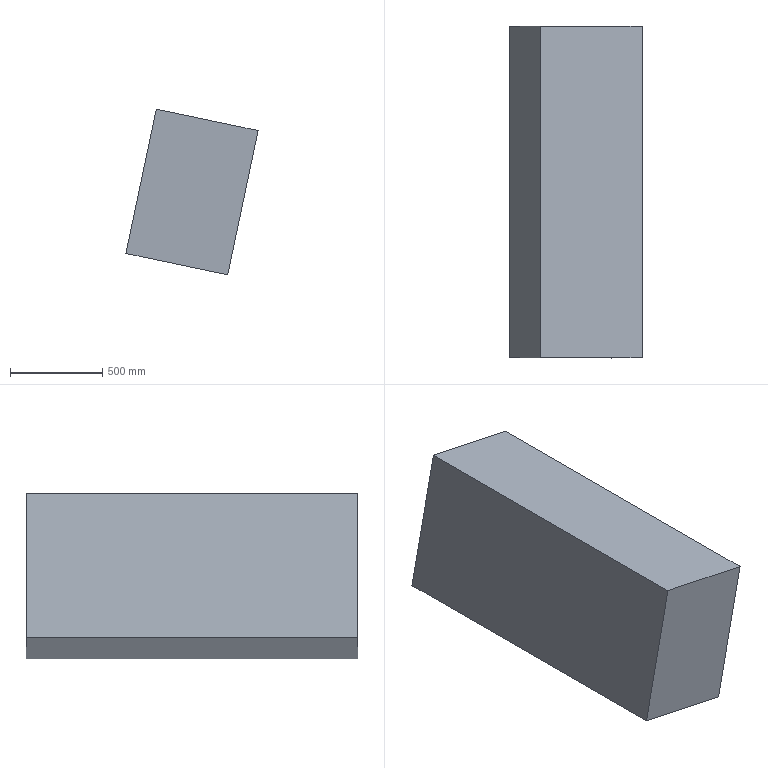Part | STEP file | 5_ESTAGIO_MAQUINA | 1 solid | 6 faces | box 717.439 x 1800 x 899.09 mm | volume 813600000 mm3 | plane 6
STEP:
#1=CARTESIAN_POINT('',(0.,0.,0.));
#2=DIRECTION('',(0.,0.,1.));
#3=DIRECTION('',(1.,0.,0.));
#4=AXIS2_PLACEMENT_3D('',#1,#2,#3);
#5=CARTESIAN_POINT('',(-2622.628,266.85,-322.944));
#6=VERTEX_POINT('',#5);
#7=CARTESIAN_POINT('',(-3175.552,266.85,-206.755));
#8=VERTEX_POINT('',#7);
#9=CARTESIAN_POINT('',(-2622.628,266.85,-322.944));
#10=DIRECTION('',(-0.9786,0.,0.2056));
#11=VECTOR('',#10,1.);
#12=LINE('',#9,#11);
#13=CARTESIAN_POINT('',(-2458.113,266.85,459.958));
#14=DIRECTION('',(0.,-1.,0.));
#15=DIRECTION('',(0.,0.,-1.));
#16=AXIS2_PLACEMENT_3D('',#13,#14,#15);
#17=PLANE('',#16);
#18=CARTESIAN_POINT('',(782.902,-164.515));
#19=DIRECTION('',(-0.2056,-0.9786));
#20=VECTOR('',#19,1.);
#21=LINE('',#18,#20);
#22=(GEOMETRIC_REPRESENTATION_CONTEXT(2)PARAMETRIC_REPRESENTATION_CONTEXT()REPRESENTATION_CONTEXT('',''));
#23=DEFINITIONAL_REPRESENTATION('',(#21),#22);
#24=PCURVE('',#17,#23);
#25=CARTESIAN_POINT('',(-175.901,0.,-837.086));
#26=DIRECTION('',(0.2056,0.,0.9786));
#27=DIRECTION('',(0.9786,0.,-0.2056));
#28=AXIS2_PLACEMENT_3D('',#25,#26,#27);
#29=PLANE('',#28);
#30=CARTESIAN_POINT('',(-2500.163,266.85));
#31=DIRECTION('',(-1.,0.));
#32=VECTOR('',#31,1.);
#33=LINE('',#30,#32);
#34=(GEOMETRIC_REPRESENTATION_CONTEXT(2)PARAMETRIC_REPRESENTATION_CONTEXT()REPRESENTATION_CONTEXT('',''));
#35=DEFINITIONAL_REPRESENTATION('',(#33),#34);
#36=PCURVE('',#29,#35);
#37=SURFACE_CURVE('',#12,(#24,#36),.PCURVE_S1.);
#38=EDGE_CURVE('',#6,#8,#37,.T.);
#39=ORIENTED_EDGE('',*,*,#38,.T.);
#40=CARTESIAN_POINT('',(-3011.037,266.85,576.146));
#41=VERTEX_POINT('',#40);
#42=CARTESIAN_POINT('',(-3011.037,266.85,576.146));
#43=DIRECTION('',(-0.2056,0.,-0.9786));
#44=VECTOR('',#43,1.);
#45=LINE('',#42,#44);
#46=CARTESIAN_POINT('',(-116.188,-552.924));
#47=DIRECTION('',(0.9786,-0.2056));
#48=VECTOR('',#47,1.);
#49=LINE('',#46,#48);
#50=(GEOMETRIC_REPRESENTATION_CONTEXT(2)PARAMETRIC_REPRESENTATION_CONTEXT()REPRESENTATION_CONTEXT('',''));
#51=DEFINITIONAL_REPRESENTATION('',(#49),#50);
#52=PCURVE('',#17,#51);
#53=CARTESIAN_POINT('',(-3011.037,-1533.15,576.146));
#54=DIRECTION('',(-0.9786,0.,0.2056));
#55=DIRECTION('',(0.2056,0.,0.9786));
#56=AXIS2_PLACEMENT_3D('',#53,#54,#55);
#57=PLANE('',#56);
#58=CARTESIAN_POINT('',(0.,1800.));
#59=DIRECTION('',(-1.,0.));
#60=VECTOR('',#59,1.);
#61=LINE('',#58,#60);
#62=(GEOMETRIC_REPRESENTATION_CONTEXT(2)PARAMETRIC_REPRESENTATION_CONTEXT()REPRESENTATION_CONTEXT('',''));
#63=DEFINITIONAL_REPRESENTATION('',(#61),#62);
#64=PCURVE('',#57,#63);
#65=SURFACE_CURVE('',#45,(#52,#64),.PCURVE_S1.);
#66=EDGE_CURVE('',#41,#8,#65,.T.);
#67=ORIENTED_EDGE('',*,*,#66,.F.);
#68=CARTESIAN_POINT('',(-2458.113,266.85,459.958));
#69=VERTEX_POINT('',#68);
#70=CARTESIAN_POINT('',(-2458.113,266.85,459.958));
#71=DIRECTION('',(-0.9786,0.,0.2056));
#72=VECTOR('',#71,1.);
#73=LINE('',#70,#72);
#74=CARTESIAN_POINT('',(0.000000001,-0.000000001));
#75=DIRECTION('',(-0.2056,-0.9786));
#76=VECTOR('',#75,1.);
#77=LINE('',#74,#76);
#78=(GEOMETRIC_REPRESENTATION_CONTEXT(2)PARAMETRIC_REPRESENTATION_CONTEXT()REPRESENTATION_CONTEXT('',''));
#79=DEFINITIONAL_REPRESENTATION('',(#77),#78);
#80=PCURVE('',#17,#79);
#81=CARTESIAN_POINT('',(-11.386,0.,-54.184));
#82=DIRECTION('',(0.2056,0.,0.9786));
#83=DIRECTION('',(0.9786,0.,-0.2056));
#84=AXIS2_PLACEMENT_3D('',#81,#82,#83);
#85=PLANE('',#84);
#86=CARTESIAN_POINT('',(-2500.163,266.85));
#87=DIRECTION('',(-1.,0.));
#88=VECTOR('',#87,1.);
#89=LINE('',#86,#88);
#90=(GEOMETRIC_REPRESENTATION_CONTEXT(2)PARAMETRIC_REPRESENTATION_CONTEXT()REPRESENTATION_CONTEXT('',''));
#91=DEFINITIONAL_REPRESENTATION('',(#89),#90);
#92=PCURVE('',#85,#91);
#93=SURFACE_CURVE('',#73,(#80,#92),.PCURVE_S1.);
#94=EDGE_CURVE('',#69,#41,#93,.T.);
#95=ORIENTED_EDGE('',*,*,#94,.F.);
#96=CARTESIAN_POINT('',(-2458.113,266.85,459.958));
#97=DIRECTION('',(-0.2056,0.,-0.9786));
#98=VECTOR('',#97,1.);
#99=LINE('',#96,#98);
#100=CARTESIAN_POINT('',(0.,-0.000000003));
#101=DIRECTION('',(0.9786,-0.2056));
#102=VECTOR('',#101,1.);
#103=LINE('',#100,#102);
#104=(GEOMETRIC_REPRESENTATION_CONTEXT(2)PARAMETRIC_REPRESENTATION_CONTEXT()REPRESENTATION_CONTEXT('',''));
#105=DEFINITIONAL_REPRESENTATION('',(#103),#104);
#106=PCURVE('',#17,#105);
#107=CARTESIAN_POINT('',(-2458.113,266.85,459.958));
#108=DIRECTION('',(0.9786,0.,-0.2056));
#109=DIRECTION('',(-0.2056,0.,-0.9786));
#110=AXIS2_PLACEMENT_3D('',#107,#108,#109);
#111=PLANE('',#110);
#112=CARTESIAN_POINT('',(0.000000001,0.));
#113=DIRECTION('',(1.,0.));
#114=VECTOR('',#113,1.);
#115=LINE('',#112,#114);
#116=(GEOMETRIC_REPRESENTATION_CONTEXT(2)PARAMETRIC_REPRESENTATION_CONTEXT()REPRESENTATION_CONTEXT('',''));
#117=DEFINITIONAL_REPRESENTATION('',(#115),#116);
#118=PCURVE('',#111,#117);
#119=SURFACE_CURVE('',#99,(#106,#118),.PCURVE_S1.);
#120=EDGE_CURVE('',#69,#6,#119,.T.);
#121=ORIENTED_EDGE('',*,*,#120,.T.);
#122=EDGE_LOOP('',(#39,#67,#95,#121));
#123=FACE_BOUND('',#122,.T.);
#124=ADVANCED_FACE('',(#123),#17,.F.);
#125=CARTESIAN_POINT('',(-3175.552,-1533.15,-206.755));
#126=VERTEX_POINT('',#125);
#127=CARTESIAN_POINT('',(-3175.552,-1533.15,-206.755));
#128=DIRECTION('',(0.,1.,0.));
#129=VECTOR('',#128,1.);
#130=LINE('',#127,#129);
#131=CARTESIAN_POINT('',(-800.,0.));
#132=DIRECTION('',(0.,1.));
#133=VECTOR('',#132,1.);
#134=LINE('',#131,#133);
#135=(GEOMETRIC_REPRESENTATION_CONTEXT(2)PARAMETRIC_REPRESENTATION_CONTEXT()REPRESENTATION_CONTEXT('',''));
#136=DEFINITIONAL_REPRESENTATION('',(#134),#135);
#137=PCURVE('',#57,#136);
#138=CARTESIAN_POINT('',(-3065.163,-1533.15));
#139=DIRECTION('',(0.,1.));
#140=VECTOR('',#139,1.);
#141=LINE('',#138,#140);
#142=(GEOMETRIC_REPRESENTATION_CONTEXT(2)PARAMETRIC_REPRESENTATION_CONTEXT()REPRESENTATION_CONTEXT('',''));
#143=DEFINITIONAL_REPRESENTATION('',(#141),#142);
#144=PCURVE('',#29,#143);
#145=SURFACE_CURVE('',#130,(#137,#144),.PCURVE_S1.);
#146=EDGE_CURVE('',#126,#8,#145,.T.);
#147=ORIENTED_EDGE('',*,*,#146,.F.);
#148=CARTESIAN_POINT('',(-3011.037,-1533.15,576.146));
#149=VERTEX_POINT('',#148);
#150=CARTESIAN_POINT('',(-3011.037,-1533.15,576.146));
#151=DIRECTION('',(-0.2056,0.,-0.9786));
#152=VECTOR('',#151,1.);
#153=LINE('',#150,#152);
#154=CARTESIAN_POINT('',(0.,0.));
#155=DIRECTION('',(-1.,0.));
#156=VECTOR('',#155,1.);
#157=LINE('',#154,#156);
#158=(GEOMETRIC_REPRESENTATION_CONTEXT(2)PARAMETRIC_REPRESENTATION_CONTEXT()REPRESENTATION_CONTEXT('',''));
#159=DEFINITIONAL_REPRESENTATION('',(#157),#158);
#160=PCURVE('',#57,#159);
#161=CARTESIAN_POINT('',(-3011.037,-1533.15,576.146));
#162=DIRECTION('',(0.,1.,0.));
#163=DIRECTION('',(0.,0.,1.));
#164=AXIS2_PLACEMENT_3D('',#161,#162,#163);
#165=PLANE('',#164);
#166=CARTESIAN_POINT('',(0.,-0.000000003));
#167=DIRECTION('',(-0.9786,-0.2056));
#168=VECTOR('',#167,1.);
#169=LINE('',#166,#168);
#170=(GEOMETRIC_REPRESENTATION_CONTEXT(2)PARAMETRIC_REPRESENTATION_CONTEXT()REPRESENTATION_CONTEXT('',''));
#171=DEFINITIONAL_REPRESENTATION('',(#169),#170);
#172=PCURVE('',#165,#171);
#173=SURFACE_CURVE('',#153,(#160,#172),.PCURVE_S1.);
#174=EDGE_CURVE('',#149,#126,#173,.T.);
#175=ORIENTED_EDGE('',*,*,#174,.F.);
#176=CARTESIAN_POINT('',(-3011.037,-1533.15,576.146));
#177=DIRECTION('',(0.,1.,0.));
#178=VECTOR('',#177,1.);
#179=LINE('',#176,#178);
#180=CARTESIAN_POINT('',(0.,0.));
#181=DIRECTION('',(0.,1.));
#182=VECTOR('',#181,1.);
#183=LINE('',#180,#182);
#184=(GEOMETRIC_REPRESENTATION_CONTEXT(2)PARAMETRIC_REPRESENTATION_CONTEXT()REPRESENTATION_CONTEXT('',''));
#185=DEFINITIONAL_REPRESENTATION('',(#183),#184);
#186=PCURVE('',#57,#185);
#187=CARTESIAN_POINT('',(-3065.163,-1533.15));
#188=DIRECTION('',(0.,1.));
#189=VECTOR('',#188,1.);
#190=LINE('',#187,#189);
#191=(GEOMETRIC_REPRESENTATION_CONTEXT(2)PARAMETRIC_REPRESENTATION_CONTEXT()REPRESENTATION_CONTEXT('',''));
#192=DEFINITIONAL_REPRESENTATION('',(#190),#191);
#193=PCURVE('',#85,#192);
#194=SURFACE_CURVE('',#179,(#186,#193),.PCURVE_S1.);
#195=EDGE_CURVE('',#149,#41,#194,.T.);
#196=ORIENTED_EDGE('',*,*,#195,.T.);
#197=ORIENTED_EDGE('',*,*,#66,.T.);
#198=EDGE_LOOP('',(#147,#175,#196,#197));
#199=FACE_BOUND('',#198,.T.);
#200=ADVANCED_FACE('',(#199),#57,.T.);
#201=CARTESIAN_POINT('',(-2622.628,-1533.15,-322.944));
#202=VERTEX_POINT('',#201);
#203=CARTESIAN_POINT('',(-3175.552,-1533.15,-206.755));
#204=DIRECTION('',(0.9786,0.,-0.2056));
#205=VECTOR('',#204,1.);
#206=LINE('',#203,#205);
#207=CARTESIAN_POINT('',(-782.902,-164.515));
#208=DIRECTION('',(-0.2056,0.9786));
#209=VECTOR('',#208,1.);
#210=LINE('',#207,#209);
#211=(GEOMETRIC_REPRESENTATION_CONTEXT(2)PARAMETRIC_REPRESENTATION_CONTEXT()REPRESENTATION_CONTEXT('',''));
#212=DEFINITIONAL_REPRESENTATION('',(#210),#211);
#213=PCURVE('',#165,#212);
#214=CARTESIAN_POINT('',(-3065.163,-1533.15));
#215=DIRECTION('',(1.,0.));
#216=VECTOR('',#215,1.);
#217=LINE('',#214,#216);
#218=(GEOMETRIC_REPRESENTATION_CONTEXT(2)PARAMETRIC_REPRESENTATION_CONTEXT()REPRESENTATION_CONTEXT('',''));
#219=DEFINITIONAL_REPRESENTATION('',(#217),#218);
#220=PCURVE('',#29,#219);
#221=SURFACE_CURVE('',#206,(#213,#220),.PCURVE_S1.);
#222=EDGE_CURVE('',#126,#202,#221,.T.);
#223=ORIENTED_EDGE('',*,*,#222,.T.);
#224=CARTESIAN_POINT('',(-2458.113,-1533.15,459.958));
#225=VERTEX_POINT('',#224);
#226=CARTESIAN_POINT('',(-2458.113,-1533.15,459.958));
#227=DIRECTION('',(-0.2056,0.,-0.9786));
#228=VECTOR('',#227,1.);
#229=LINE('',#226,#228);
#230=CARTESIAN_POINT('',(-116.188,552.924));
#231=DIRECTION('',(-0.9786,-0.2056));
#232=VECTOR('',#231,1.);
#233=LINE('',#230,#232);
#234=(GEOMETRIC_REPRESENTATION_CONTEXT(2)PARAMETRIC_REPRESENTATION_CONTEXT()REPRESENTATION_CONTEXT('',''));
#235=DEFINITIONAL_REPRESENTATION('',(#233),#234);
#236=PCURVE('',#165,#235);
#237=CARTESIAN_POINT('',(0.000000001,-1800.));
#238=DIRECTION('',(1.,0.));
#239=VECTOR('',#238,1.);
#240=LINE('',#237,#239);
#241=(GEOMETRIC_REPRESENTATION_CONTEXT(2)PARAMETRIC_REPRESENTATION_CONTEXT()REPRESENTATION_CONTEXT('',''));
#242=DEFINITIONAL_REPRESENTATION('',(#240),#241);
#243=PCURVE('',#111,#242);
#244=SURFACE_CURVE('',#229,(#236,#243),.PCURVE_S1.);
#245=EDGE_CURVE('',#225,#202,#244,.T.);
#246=ORIENTED_EDGE('',*,*,#245,.F.);
#247=CARTESIAN_POINT('',(-3011.037,-1533.15,576.146));
#248=DIRECTION('',(0.9786,0.,-0.2056));
#249=VECTOR('',#248,1.);
#250=LINE('',#247,#249);
#251=CARTESIAN_POINT('',(-0.000000001,-0.000000001));
#252=DIRECTION('',(-0.2056,0.9786));
#253=VECTOR('',#252,1.);
#254=LINE('',#251,#253);
#255=(GEOMETRIC_REPRESENTATION_CONTEXT(2)PARAMETRIC_REPRESENTATION_CONTEXT()REPRESENTATION_CONTEXT('',''));
#256=DEFINITIONAL_REPRESENTATION('',(#254),#255);
#257=PCURVE('',#165,#256);
#258=CARTESIAN_POINT('',(-3065.163,-1533.15));
#259=DIRECTION('',(1.,0.));
#260=VECTOR('',#259,1.);
#261=LINE('',#258,#260);
#262=(GEOMETRIC_REPRESENTATION_CONTEXT(2)PARAMETRIC_REPRESENTATION_CONTEXT()REPRESENTATION_CONTEXT('',''));
#263=DEFINITIONAL_REPRESENTATION('',(#261),#262);
#264=PCURVE('',#85,#263);
#265=SURFACE_CURVE('',#250,(#257,#264),.PCURVE_S1.);
#266=EDGE_CURVE('',#149,#225,#265,.T.);
#267=ORIENTED_EDGE('',*,*,#266,.F.);
#268=ORIENTED_EDGE('',*,*,#174,.T.);
#269=EDGE_LOOP('',(#223,#246,#267,#268));
#270=FACE_BOUND('',#269,.T.);
#271=ADVANCED_FACE('',(#270),#165,.F.);
#272=CARTESIAN_POINT('',(-2622.628,266.85,-322.944));
#273=DIRECTION('',(0.,-1.,0.));
#274=VECTOR('',#273,1.);
#275=LINE('',#272,#274);
#276=CARTESIAN_POINT('',(800.,0.));
#277=DIRECTION('',(0.,-1.));
#278=VECTOR('',#277,1.);
#279=LINE('',#276,#278);
#280=(GEOMETRIC_REPRESENTATION_CONTEXT(2)PARAMETRIC_REPRESENTATION_CONTEXT()REPRESENTATION_CONTEXT('',''));
#281=DEFINITIONAL_REPRESENTATION('',(#279),#280);
#282=PCURVE('',#111,#281);
#283=CARTESIAN_POINT('',(-2500.163,266.85));
#284=DIRECTION('',(0.,-1.));
#285=VECTOR('',#284,1.);
#286=LINE('',#283,#285);
#287=(GEOMETRIC_REPRESENTATION_CONTEXT(2)PARAMETRIC_REPRESENTATION_CONTEXT()REPRESENTATION_CONTEXT('',''));
#288=DEFINITIONAL_REPRESENTATION('',(#286),#287);
#289=PCURVE('',#29,#288);
#290=SURFACE_CURVE('',#275,(#282,#289),.PCURVE_S1.);
#291=EDGE_CURVE('',#6,#202,#290,.T.);
#292=ORIENTED_EDGE('',*,*,#291,.F.);
#293=ORIENTED_EDGE('',*,*,#120,.F.);
#294=CARTESIAN_POINT('',(-2458.113,266.85,459.958));
#295=DIRECTION('',(0.,-1.,0.));
#296=VECTOR('',#295,1.);
#297=LINE('',#294,#296);
#298=CARTESIAN_POINT('',(0.,0.));
#299=DIRECTION('',(0.,-1.));
#300=VECTOR('',#299,1.);
#301=LINE('',#298,#300);
#302=(GEOMETRIC_REPRESENTATION_CONTEXT(2)PARAMETRIC_REPRESENTATION_CONTEXT()REPRESENTATION_CONTEXT('',''));
#303=DEFINITIONAL_REPRESENTATION('',(#301),#302);
#304=PCURVE('',#111,#303);
#305=CARTESIAN_POINT('',(-2500.163,266.85));
#306=DIRECTION('',(0.,-1.));
#307=VECTOR('',#306,1.);
#308=LINE('',#305,#307);
#309=(GEOMETRIC_REPRESENTATION_CONTEXT(2)PARAMETRIC_REPRESENTATION_CONTEXT()REPRESENTATION_CONTEXT('',''));
#310=DEFINITIONAL_REPRESENTATION('',(#308),#309);
#311=PCURVE('',#85,#310);
#312=SURFACE_CURVE('',#297,(#304,#311),.PCURVE_S1.);
#313=EDGE_CURVE('',#69,#225,#312,.T.);
#314=ORIENTED_EDGE('',*,*,#313,.T.);
#315=ORIENTED_EDGE('',*,*,#245,.T.);
#316=EDGE_LOOP('',(#292,#293,#314,#315));
#317=FACE_BOUND('',#316,.T.);
#318=ADVANCED_FACE('',(#317),#111,.T.);
#319=ORIENTED_EDGE('',*,*,#94,.T.);
#320=ORIENTED_EDGE('',*,*,#195,.F.);
#321=ORIENTED_EDGE('',*,*,#266,.T.);
#322=ORIENTED_EDGE('',*,*,#313,.F.);
#323=EDGE_LOOP('',(#319,#320,#321,#322));
#324=FACE_BOUND('',#323,.T.);
#325=ADVANCED_FACE('',(#324),#85,.T.);
#326=ORIENTED_EDGE('',*,*,#291,.T.);
#327=ORIENTED_EDGE('',*,*,#222,.F.);
#328=ORIENTED_EDGE('',*,*,#146,.T.);
#329=ORIENTED_EDGE('',*,*,#38,.F.);
#330=EDGE_LOOP('',(#326,#327,#328,#329));
#331=FACE_BOUND('',#330,.T.);
#332=ADVANCED_FACE('',(#331),#29,.F.);
#333=CLOSED_SHELL('',(#124,#200,#271,#318,#325,#332));
#334=MANIFOLD_SOLID_BREP('',#333);
#335=(LENGTH_UNIT()NAMED_UNIT(*)SI_UNIT(.MILLI.,.METRE.));
#336=UNCERTAINTY_MEASURE_WITH_UNIT(LENGTH_MEASURE(0.0000001),#335,'','');
#337=(NAMED_UNIT(*)PLANE_ANGLE_UNIT()SI_UNIT($,.RADIAN.));
#338=(NAMED_UNIT(*)SI_UNIT($,.STERADIAN.)SOLID_ANGLE_UNIT());
#339=(GEOMETRIC_REPRESENTATION_CONTEXT(3)GLOBAL_UNCERTAINTY_ASSIGNED_CONTEXT((#336))GLOBAL_UNIT_ASSIGNED_CONTEXT((#335,#337,#338))REPRESENTATION_CONTEXT('',''));
#340=ADVANCED_BREP_SHAPE_REPRESENTATION('',(#4,#334),#339);